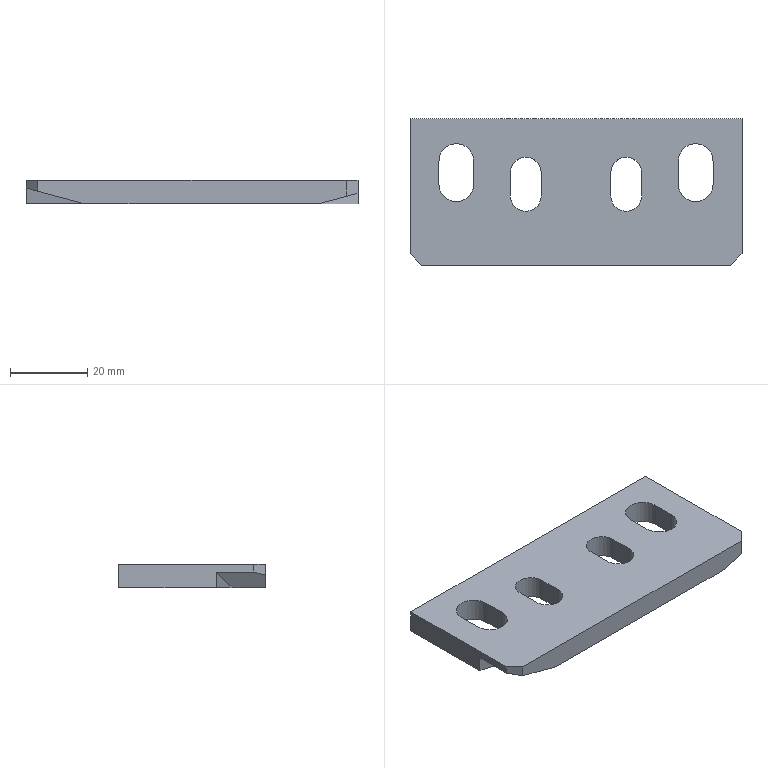Part | STEP file | gslz 2016.10.28-13_id670_x_t | 1 solid | 29 faces | box 86 x 38 x 6 mm | volume 16491 mm3 | plane 21 | cylinder 8 | commonest cylinder face diameters 8 x4 9 x4